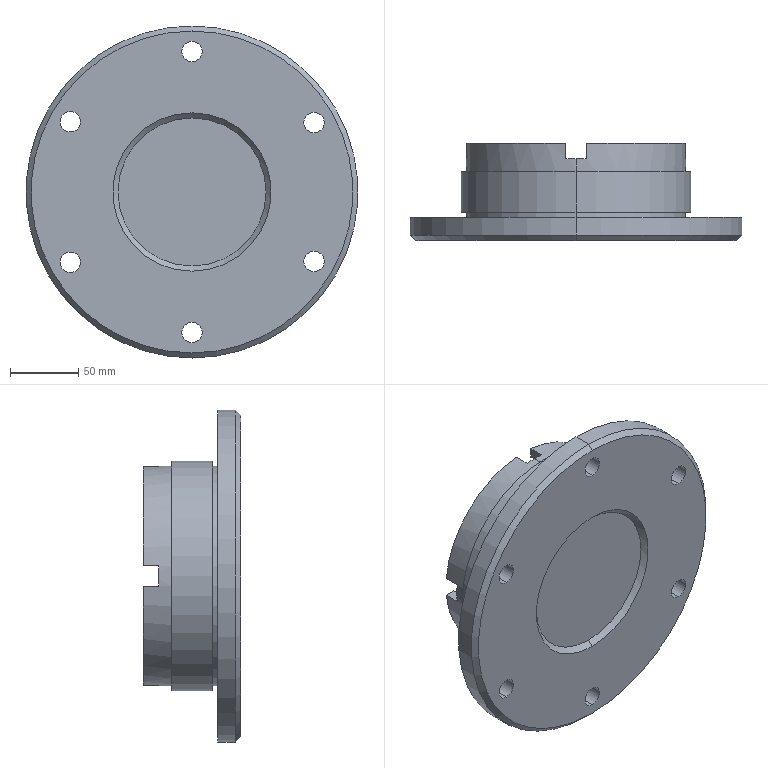Part | SolidWorks | features ICE 2, Chamfer 1, Revolution 1, Scale 1 | 1 solid | 50 faces | box 243.75 x 71.25 x 243.75 mm | volume 1137099 mm3 | plane 22 | cylinder 20 | cone 6 | torus 2 | commonest cylinder face diameters 15 x12 161.25 x4 168.75 x2 243.75 x2